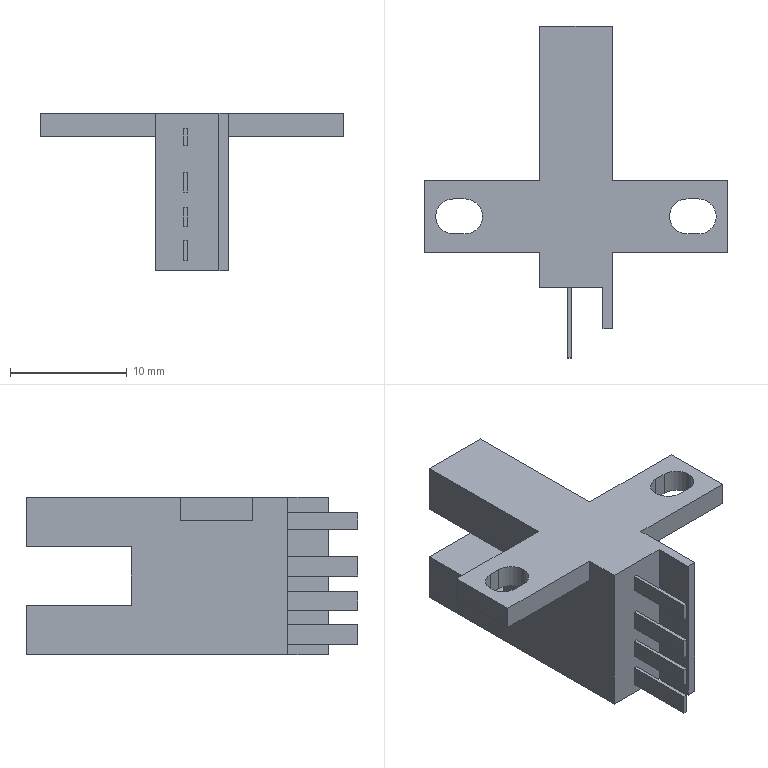Part | STEP file | SM140A-20-1140D-140A-600ABSR | 1 solid | 50 faces | box 26 x 28.4 x 13.5 mm | volume 1855 mm3 | plane 44 | cylinder 6 | commonest cylinder face diameters 3 x6